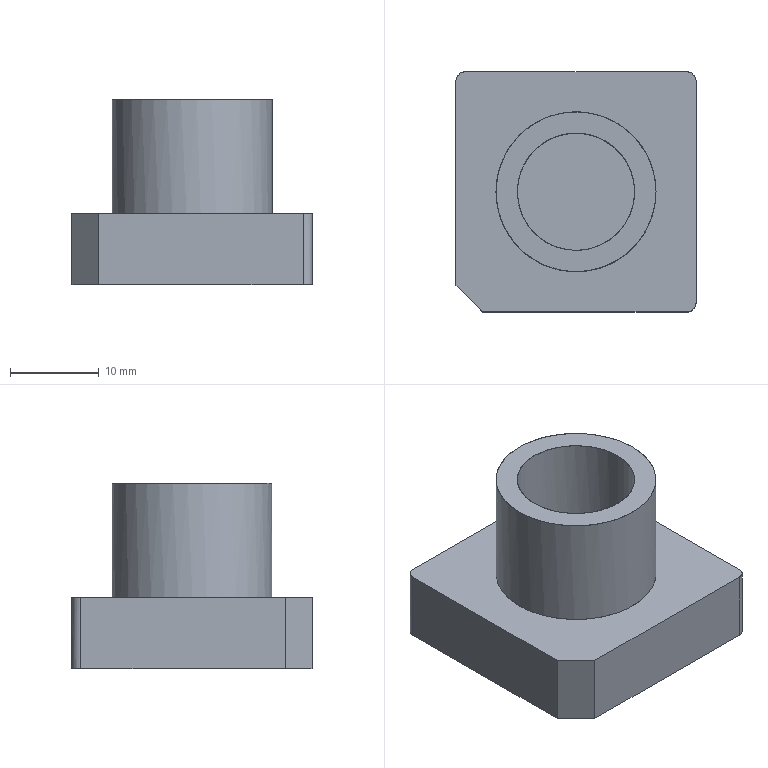NC program | PowerMill | posted with a generic post | part box 27 x 27 x 20.913 mm
Lines 16767 to 17771 of 92133:
N16864 M6
N16865 S18000 M03
N16866 G00 G90 X0.0 Y0.0
N16867 G43 Z10.803 H14
N16868
N16869 G05 P10000 R8
N16870 X-0.5036 Y-4.0685
N16871 Z0.9259
N16872 G01 Z-0.2741 F1200.0
N16873 X-0.499 Y-4.1188 F2000.0
N16874 X-0.4906 Y-4.1686
N16875 X-0.4782 Y-4.2176
N16876 X-0.4619 Y-4.2654
N16877 X-0.442 Y-4.3119
N16878 X-0.4184 Y-4.3566
N16879 X-0.3914 Y-4.3994
N16880 X-0.3611 Y-4.4398
N16881 X-0.3278 Y-4.4777
N16882 X-0.2915 Y-4.5129
N16883 X-0.2526 Y-4.5451
N16884 X-0.2112 Y-4.5741
N16885 X-0.1677 Y-4.5998
N16886 X-0.1223 Y-4.622
N16887 X-0.0753 Y-4.6405
N16888 X-0.0269 Y-4.6553
N16889 X0.0224 Y-4.6662
N16890 X0.0724 Y-4.6732
N16891 X0.1229 Y-4.6762
N16892 X0.1678 Y-4.6755
N16893 X0.3042 Y-4.6686
N16894 X0.4399 Y-4.6578
N16895 X0.5751 Y-4.6431
N16896 X0.7098 Y-4.6244
N16897 X0.8439 Y-4.6018
N16898 X0.9775 Y-4.5752
N16899 X1.1107 Y-4.5447
N16900 X1.2433 Y-4.5103
N16901 X1.3744 Y-4.4722
N16902 X1.504 Y-4.4304
N16903 X1.6321 Y-4.3849
N16904 X1.7586 Y-4.3357
N16905 X1.8838 Y-4.2828
N16906 X2.0074 Y-4.2262
N16907 X2.1296 Y-4.1658
N16908 X2.2504 Y-4.1017
N16909 X2.3698 Y-4.0338
N16910 X2.4859 Y-3.9634
N16911 X2.6001 Y-3.8896
N16912 X2.7121 Y-3.8123
N16913 X2.8221 Y-3.7317
N16914 X2.9297 Y-3.6477
N16915 X3.0351 Y-3.5606
N16916 X3.138 Y-3.4702
N16917 X3.2383 Y-3.3768
N16918 X3.336 Y-3.2804
N16919 X3.4271 Y-3.1851
N16920 X3.5154 Y-3.0873
N16921 X3.602 Y-2.9857
N16922 X3.6878 Y-2.8789
N16923 X3.7713 Y-2.7688
N16924 X3.8501 Y-2.6583
N16925 X3.9235 Y-2.5489
N16926 X3.9937 Y-2.4375
N16927 X4.0634 Y-2.3194
N16928 X4.1295 Y-2.1994
N16929 X4.1921 Y-2.0775
N16930 X4.2511 Y-1.9539
N16931 X4.3064 Y-1.8287
N16932 X4.3581 Y-1.7019
N16933 X4.406 Y-1.5738
N16934 X4.4501 Y-1.4444
N16935 X4.4904 Y-1.3139
N16936 X4.5268 Y-1.1823
N16937 X4.5593 Y-1.0497
N16938 X4.5879 Y-0.9167
N16939 X4.6126 Y-0.7825
N16940 X4.6335 Y-0.6472
N16941 X4.6505 Y-0.511
N16942 X4.6635 Y-0.3744
N16943 X4.6725 Y-0.2377
N16944 X4.6775 Y-0.1012
N16945 X4.6785 Y0.0348
N16946 X4.6755 Y0.17
N16947 X4.6686 Y0.305
N16948 X4.6576 Y0.4417
N16949 X4.6426 Y0.578
N16950 X4.6237 Y0.7137
N16951 X4.6009 Y0.8488
N16952 X4.5742 Y0.9828
N16953 X4.5436 Y1.1159
N16954 X4.5091 Y1.248
N16955 X4.4708 Y1.3791
N16956 X4.4286 Y1.5091
N16957 X4.3827 Y1.6378
N16958 X4.3329 Y1.7651
N16959 X4.2795 Y1.891
N16960 X4.2224 Y2.0152
N16961 X4.1617 Y2.1378
N16962 X4.0974 Y2.2585
N16963 X4.0297 Y2.3773
N16964 X3.9586 Y2.4938
N16965 X3.8841 Y2.6083
N16966 X3.8063 Y2.7205
N16967 X3.7252 Y2.8306
N16968 X3.6408 Y2.9383
N16969 X3.5533 Y3.0435
N16970 X3.4626 Y3.1463
N16971 X3.369 Y3.2464
N16972 X3.2723 Y3.3438
N16973 X3.1772 Y3.4344
N16974 X3.0795 Y3.5223
N16975 X2.9771 Y3.6091
N16976 X2.8699 Y3.6949
N16977 X2.76 Y3.7778
N16978 X2.6498 Y3.8559
N16979 X2.5406 Y3.9289
N16980 X2.4292 Y3.9986
N16981 X2.3103 Y4.0684
N16982 X2.1898 Y4.1345
N16983 X2.0678 Y4.1968
N16984 X1.9444 Y4.2555
N16985 X1.8195 Y4.3104
N16986 X1.6931 Y4.3616
N16987 X1.5654 Y4.409
N16988 X1.4363 Y4.4527
N16989 X1.3058 Y4.4927
N16990 X1.1741 Y4.5288
N16991 X1.041 Y4.5612
N16992 X0.9074 Y4.5897
N16993 X0.7728 Y4.6142
N16994 X0.6376 Y4.6349
N16995 X0.5019 Y4.6515
N16996 X0.3657 Y4.6642
N16997 X0.2293 Y4.6729
N16998 X0.0926 Y4.6776
N16999 X-0.0442 Y4.6783
N17000 X-0.1809 Y4.675
N17001 X-0.3175 Y4.6677
N17002 X-0.4538 Y4.6565
N17003 X-0.5897 Y4.6412
N17004 X-0.7251 Y4.622
N17005 X-0.8599 Y4.5988
N17006 X-0.9938 Y4.5717
N17007 X-1.1274 Y4.5406
N17008 X-1.2597 Y4.5058
N17009 X-1.3907 Y4.4672
N17010 X-1.5203 Y4.4248
N17011 X-1.6485 Y4.3787
N17012 X-1.7753 Y4.3288
N17013 X-1.9006 Y4.2753
N17014 X-2.0245 Y4.218
N17015 X-2.1468 Y4.157
N17016 X-2.2675 Y4.0923
N17017 X-2.3866 Y4.024
N17018 X-2.5027 Y3.9529
N17019 X-2.6166 Y3.8785
N17020 X-2.7285 Y3.8006
N17021 X-2.8382 Y3.7194
N17022 X-2.9456 Y3.635
N17023 X-3.0506 Y3.5473
N17024 X-3.1531 Y3.4565
N17025 X-3.253 Y3.3626
N17026 X-3.3503 Y3.2658
N17027 X-3.4409 Y3.1702
N17028 X-3.5288 Y3.072
N17029 X-3.6159 Y2.9688
N17030 X-3.7016 Y2.8613
N17031 X-3.784 Y2.7515
N17032 X-3.8619 Y2.6412
N17033 X-3.9347 Y2.5315
N17034 X-4.0043 Y2.4196
N17035 X-4.0739 Y2.3004
N17036 X-4.1397 Y2.1799
N17037 X-4.2017 Y2.058
N17038 X-4.26 Y1.9347
N17039 X-4.3145 Y1.8099
N17040 X-4.3653 Y1.6838
N17041 X-4.4123 Y1.5563
N17042 X-4.4556 Y1.4273
N17043 X-4.4952 Y1.2969
N17044 X-4.5311 Y1.165
N17045 X-4.5628 Y1.0335
N17046 X-4.5908 Y0.9014
N17047 X-4.615 Y0.7685
N17048 X-4.6354 Y0.6347
N17049 X-4.6517 Y0.5003
N17050 X-4.6642 Y0.3656
N17051 X-4.6727 Y0.2308
N17052 X-4.6775 Y0.0953
N17053 X-4.6783 Y-0.0414
N17054 X-4.6752 Y-0.1778
N17055 X-4.6681 Y-0.3138
N17056 X-4.657 Y-0.4494
N17057 X-4.6419 Y-0.5846
N17058 X-4.6229 Y-0.7196
N17059 X-4.5998 Y-0.8542
N17060 X-4.5728 Y-0.9885
N17061 X-4.5418 Y-1.1222
N17062 X-4.5071 Y-1.2546
N17063 X-4.4688 Y-1.3855
N17064 X-4.4267 Y-1.5149
N17065 X-4.3809 Y-1.6428
N17066 X-4.3314 Y-1.7693
N17067 X-4.2781 Y-1.8944
N17068 X-4.2211 Y-2.018
N17069 X-4.1604 Y-2.1401
N17070 X-4.0959 Y-2.2609
N17071 X-4.0277 Y-2.3803
N17072 X-3.957 Y-2.4962
N17073 X-3.8828 Y-2.6102
N17074 X-3.8052 Y-2.7221
N17075 X-3.7243 Y-2.8318
N17076 X-3.6401 Y-2.9393
N17077 X-3.5526 Y-3.0444
N17078 X-3.462 Y-3.147
N17079 X-3.3683 Y-3.2471
N17080 X-3.2716 Y-3.3445
N17081 X-3.1758 Y-3.4357
N17082 X-3.0774 Y-3.5241
N17083 X-2.9748 Y-3.611
N17084 X-2.8675 Y-3.6967
N17085 X-2.7573 Y-3.7797
N17086 X-2.6468 Y-3.8581
N17087 X-2.5367 Y-3.9314
N17088 X-2.4246 Y-4.0015
N17089 X-2.3063 Y-4.0708
N17090 X-2.1861 Y-4.1365
N17091 X-2.0641 Y-4.1987
N17092 X-1.9403 Y-4.2573
N17093 X-1.8149 Y-4.3123
N17094 X-1.6881 Y-4.3635
N17095 X-1.5598 Y-4.411
N17096 X-1.4303 Y-4.4546
N17097 X-1.2997 Y-4.4945
N17098 X-1.168 Y-4.5305
N17099 X-1.0353 Y-4.5626
N17100 X-0.9018 Y-4.5908
N17101 X-0.767 Y-4.6152
N17102 X-0.6316 Y-4.6357
N17103 X-0.4957 Y-4.6522
N17104 X-0.3595 Y-4.6647
N17105 X-0.223 Y-4.6732
N17106 X-0.0863 Y-4.6777
N17107 X0.0503 Y-4.6782
N17108 X0.1678 Y-4.6755
N17109 X0.2182 Y-4.6723
N17110 X0.2683 Y-4.6652
N17111 X0.3176 Y-4.6541
N17112 X0.3658 Y-4.6392
N17113 X0.4128 Y-4.6205
N17114 X0.4582 Y-4.5981
N17115 X0.5016 Y-4.5723
N17116 X0.5428 Y-4.5431
N17117 X0.5816 Y-4.5108
N17118 X0.6178 Y-4.4754
N17119 X0.651 Y-4.4374
N17120 X0.6812 Y-4.3969
N17121 X0.708 Y-4.3541
N17122 X0.7314 Y-4.3093
N17123 X0.7512 Y-4.2627
N17124 X0.7673 Y-4.2148
N17125 X0.7795 Y-4.1658
N17126 X0.7878 Y-4.116
N17127 X0.7921 Y-4.0656
N17128 X0.7927 Y-4.0207
N17129 X-0.5036 Y-4.0685 Z-0.314
N17130 X-0.499 Y-4.1188
N17131 X-0.4906 Y-4.1686
N17132 X-0.4782 Y-4.2176
N17133 X-0.4619 Y-4.2654
N17134 X-0.442 Y-4.3119
N17135 X-0.4184 Y-4.3566
N17136 X-0.3914 Y-4.3994
N17137 X-0.3611 Y-4.4398
N17138 X-0.3278 Y-4.4777
N17139 X-0.2915 Y-4.5129
N17140 X-0.2526 Y-4.5451
N17141 X-0.2112 Y-4.5741
N17142 X-0.1677 Y-4.5998
N17143 X-0.1223 Y-4.622
N17144 X-0.0753 Y-4.6405
N17145 X-0.0269 Y-4.6553
N17146 X0.0224 Y-4.6662
N17147 X0.0724 Y-4.6732
N17148 X0.1229 Y-4.6762
N17149 X0.1678 Y-4.6755
N17150 X0.3042 Y-4.6686
N17151 X0.4399 Y-4.6578
N17152 X0.5751 Y-4.6431
N17153 X0.7098 Y-4.6244
N17154 X0.8439 Y-4.6018
N17155 X0.9775 Y-4.5752
N17156 X1.1107 Y-4.5447
N17157 X1.2433 Y-4.5103
N17158 X1.3744 Y-4.4722
N17159 X1.504 Y-4.4304
N17160 X1.6321 Y-4.3849
N17161 X1.7586 Y-4.3357
N17162 X1.8838 Y-4.2828
N17163 X2.0074 Y-4.2262
N17164 X2.1296 Y-4.1658
N17165 X2.2504 Y-4.1017
N17166 X2.3698 Y-4.0338
N17167 X2.4859 Y-3.9634
N17168 X2.6001 Y-3.8896
N17169 X2.7121 Y-3.8123
N17170 X2.8221 Y-3.7317
N17171 X2.9297 Y-3.6477
N17172 X3.0351 Y-3.5606
N17173 X3.138 Y-3.4702
N17174 X3.2383 Y-3.3768
N17175 X3.336 Y-3.2803
N17176 X3.4271 Y-3.1851
N17177 X3.5154 Y-3.0873
N17178 X3.602 Y-2.9857
N17179 X3.6878 Y-2.8789
N17180 X3.7713 Y-2.7688
N17181 X3.8501 Y-2.6583
N17182 X3.9235 Y-2.5489
N17183 X3.9937 Y-2.4375
N17184 X4.0634 Y-2.3194
N17185 X4.1295 Y-2.1994
N17186 X4.1921 Y-2.0775
N17187 X4.2511 Y-1.9539
N17188 X4.3064 Y-1.8287
N17189 X4.3581 Y-1.7019
N17190 X4.406 Y-1.5738
N17191 X4.4501 Y-1.4444
N17192 X4.4904 Y-1.3139
N17193 X4.5268 Y-1.1823
N17194 X4.5593 Y-1.0497
N17195 X4.5879 Y-0.9167
N17196 X4.6126 Y-0.7825
N17197 X4.6335 Y-0.6472
N17198 X4.6505 Y-0.511
N17199 X4.6635 Y-0.3744
N17200 X4.6725 Y-0.2377
N17201 X4.6775 Y-0.1012
N17202 X4.6785 Y0.0348
N17203 X4.6755 Y0.17
N17204 X4.6686 Y0.305
N17205 X4.6576 Y0.4417
N17206 X4.6426 Y0.578
N17207 X4.6237 Y0.7137
N17208 X4.6009 Y0.8488
N17209 X4.5742 Y0.9828
N17210 X4.5436 Y1.1159
N17211 X4.5091 Y1.248
N17212 X4.4708 Y1.3791
N17213 X4.4286 Y1.5091
N17214 X4.3827 Y1.6378
N17215 X4.3329 Y1.7651
N17216 X4.2795 Y1.891
N17217 X4.2224 Y2.0152
N17218 X4.1617 Y2.1378
N17219 X4.0974 Y2.2585
N17220 X4.0297 Y2.3773
N17221 X3.9586 Y2.4938
N17222 X3.8841 Y2.6083
N17223 X3.8063 Y2.7205
N17224 X3.7252 Y2.8306
N17225 X3.6408 Y2.9383
N17226 X3.5533 Y3.0435
N17227 X3.4626 Y3.1463
N17228 X3.369 Y3.2464
N17229 X3.2723 Y3.3438
N17230 X3.1772 Y3.4345
N17231 X3.0795 Y3.5223
N17232 X2.9771 Y3.6091
N17233 X2.8699 Y3.6949
N17234 X2.76 Y3.7778
N17235 X2.6498 Y3.856
N17236 X2.5405 Y3.9289
N17237 X2.4292 Y3.9986
N17238 X2.3102 Y4.0684
N17239 X2.1898 Y4.1345
N17240 X2.0678 Y4.1969
N17241 X1.9443 Y4.2555
N17242 X1.8194 Y4.3104
N17243 X1.6931 Y4.3616
N17244 X1.5654 Y4.4091
N17245 X1.4363 Y4.4527
N17246 X1.3058 Y4.4927
N17247 X1.174 Y4.5288
N17248 X1.0409 Y4.5612
N17249 X0.9073 Y4.5897
N17250 X0.7728 Y4.6142
N17251 X0.6376 Y4.6349
N17252 X0.5019 Y4.6515
N17253 X0.3657 Y4.6642
N17254 X0.2292 Y4.6729
N17255 X0.0925 Y4.6776
N17256 X-0.0442 Y4.6783
N17257 X-0.1809 Y4.675
N17258 X-0.3175 Y4.6677
N17259 X-0.4538 Y4.6565
N17260 X-0.5897 Y4.6412
N17261 X-0.7251 Y4.622
N17262 X-0.8599 Y4.5988
N17263 X-0.9938 Y4.5717
N17264 X-1.1274 Y4.5406
N17265 X-1.2597 Y4.5058
N17266 X-1.3907 Y4.4672
N17267 X-1.5204 Y4.4248
N17268 X-1.6486 Y4.3787
N17269 X-1.7754 Y4.3288
N17270 X-1.9007 Y4.2752
N17271 X-2.0245 Y4.218
N17272 X-2.1468 Y4.157
N17273 X-2.2675 Y4.0923
N17274 X-2.3867 Y4.024
N17275 X-2.5027 Y3.9529
N17276 X-2.6167 Y3.8785
N17277 X-2.7285 Y3.8006
N17278 X-2.8382 Y3.7194
N17279 X-2.9456 Y3.6349
N17280 X-3.0506 Y3.5473
N17281 X-3.1531 Y3.4564
N17282 X-3.253 Y3.3626
N17283 X-3.3503 Y3.2658
N17284 X-3.4409 Y3.1702
N17285 X-3.5288 Y3.072
N17286 X-3.616 Y2.9688
N17287 X-3.7016 Y2.8613
N17288 X-3.784 Y2.7514
N17289 X-3.8619 Y2.6412
N17290 X-3.9347 Y2.5314
N17291 X-4.0044 Y2.4196
N17292 X-4.0739 Y2.3004
N17293 X-4.1397 Y2.1799
N17294 X-4.2017 Y2.0579
N17295 X-4.26 Y1.9346
N17296 X-4.3145 Y1.8099
N17297 X-4.3653 Y1.6838
N17298 X-4.4123 Y1.5562
N17299 X-4.4556 Y1.4273
N17300 X-4.4952 Y1.2969
N17301 X-4.5311 Y1.165
N17302 X-4.5628 Y1.0335
N17303 X-4.5908 Y0.9014
N17304 X-4.615 Y0.7684
N17305 X-4.6354 Y0.6346
N17306 X-4.6517 Y0.5003
N17307 X-4.6642 Y0.3656
N17308 X-4.6727 Y0.2307
N17309 X-4.6775 Y0.0953
N17310 X-4.6783 Y-0.0414
N17311 X-4.6752 Y-0.1778
N17312 X-4.6681 Y-0.3138
N17313 X-4.657 Y-0.4494
N17314 X-4.6419 Y-0.5847
N17315 X-4.6229 Y-0.7196
N17316 X-4.5998 Y-0.8542
N17317 X-4.5728 Y-0.9885
N17318 X-4.5418 Y-1.1223
N17319 X-4.5071 Y-1.2546
N17320 X-4.4688 Y-1.3855
N17321 X-4.4267 Y-1.5149
N17322 X-4.3809 Y-1.6428
N17323 X-4.3313 Y-1.7693
N17324 X-4.2781 Y-1.8944
N17325 X-4.2211 Y-2.018
N17326 X-4.1604 Y-2.1402
N17327 X-4.0959 Y-2.2609
N17328 X-4.0277 Y-2.3803
N17329 X-3.957 Y-2.4962
N17330 X-3.8828 Y-2.6102
N17331 X-3.8052 Y-2.7221
N17332 X-3.7243 Y-2.8318
N17333 X-3.6401 Y-2.9393
N17334 X-3.5526 Y-3.0444
N17335 X-3.462 Y-3.147
N17336 X-3.3683 Y-3.2471
N17337 X-3.2716 Y-3.3446
N17338 X-3.1758 Y-3.4357
N17339 X-3.0774 Y-3.5241
N17340 X-2.9748 Y-3.611
N17341 X-2.8675 Y-3.6967
N17342 X-2.7573 Y-3.7797
N17343 X-2.6467 Y-3.8581
N17344 X-2.5367 Y-3.9314
N17345 X-2.4245 Y-4.0016
N17346 X-2.3063 Y-4.0708
N17347 X-2.1861 Y-4.1366
N17348 X-2.064 Y-4.1988
N17349 X-1.9403 Y-4.2574
N17350 X-1.8149 Y-4.3123
N17351 X-1.688 Y-4.3635
N17352 X-1.5598 Y-4.411
N17353 X-1.4303 Y-4.4546
N17354 X-1.2997 Y-4.4945
N17355 X-1.168 Y-4.5305
N17356 X-1.0353 Y-4.5626
N17357 X-0.9017 Y-4.5908
N17358 X-0.767 Y-4.6152
N17359 X-0.6316 Y-4.6357
N17360 X-0.4957 Y-4.6522
N17361 X-0.3594 Y-4.6647
N17362 X-0.2229 Y-4.6732
N17363 X-0.0863 Y-4.6777
N17364 X0.0504 Y-4.6782
N17365 X0.1678 Y-4.6755
N17366 X0.2182 Y-4.6723
N17367 X0.2683 Y-4.6652
N17368 X0.3176 Y-4.6541
N17369 X0.3658 Y-4.6392
N17370 X0.4128 Y-4.6205
N17371 X0.4582 Y-4.5981
N17372 X0.5016 Y-4.5723
N17373 X0.5428 Y-4.5431
N17374 X0.5816 Y-4.5108
N17375 X0.6178 Y-4.4754
N17376 X0.651 Y-4.4374
N17377 X0.6812 Y-4.3969
N17378 X0.708 Y-4.3541
N17379 X0.7314 Y-4.3093
N17380 X0.7512 Y-4.2627
N17381 X0.7672 Y-4.2148
N17382 X0.7795 Y-4.1658
N17383 X0.7878 Y-4.116
N17384 X0.7921 Y-4.0656
N17385 X0.7927 Y-4.0207
N17386 X-0.5036 Y-4.0685 Z-0.3539
N17387 X-0.499 Y-4.1188
N17388 X-0.4906 Y-4.1686
N17389 X-0.4782 Y-4.2176
N17390 X-0.4619 Y-4.2654
N17391 X-0.442 Y-4.3119
N17392 X-0.4184 Y-4.3566
N17393 X-0.3914 Y-4.3994
N17394 X-0.3611 Y-4.4398
N17395 X-0.3278 Y-4.4777
N17396 X-0.2915 Y-4.5129
N17397 X-0.2526 Y-4.5451
N17398 X-0.2112 Y-4.5741
N17399 X-0.1677 Y-4.5998
N17400 X-0.1223 Y-4.622
N17401 X-0.0753 Y-4.6405
N17402 X-0.0269 Y-4.6553
N17403 X0.0224 Y-4.6662
N17404 X0.0724 Y-4.6732
N17405 X0.1229 Y-4.6762
N17406 X0.1678 Y-4.6755
N17407 X0.3042 Y-4.6686
N17408 X0.4399 Y-4.6578
N17409 X0.5751 Y-4.6431
N17410 X0.7098 Y-4.6244
N17411 X0.8439 Y-4.6018
N17412 X0.9775 Y-4.5752
N17413 X1.1107 Y-4.5447
N17414 X1.2433 Y-4.5103
N17415 X1.3744 Y-4.4722
N17416 X1.504 Y-4.4304
N17417 X1.6321 Y-4.3849
N17418 X1.7587 Y-4.3357
N17419 X1.8838 Y-4.2828
N17420 X2.0074 Y-4.2262
N17421 X2.1296 Y-4.1658
N17422 X2.2504 Y-4.1017
N17423 X2.3699 Y-4.0338
N17424 X2.4859 Y-3.9634
N17425 X2.6001 Y-3.8896
N17426 X2.7122 Y-3.8123
N17427 X2.8221 Y-3.7317
N17428 X2.9298 Y-3.6477
N17429 X3.0351 Y-3.5606
N17430 X3.138 Y-3.4702
N17431 X3.2383 Y-3.3768
N17432 X3.336 Y-3.2803
N17433 X3.4271 Y-3.1851
N17434 X3.5154 Y-3.0873
N17435 X3.602 Y-2.9857
N17436 X3.6878 Y-2.8789
N17437 X3.7713 Y-2.7688
N17438 X3.8501 Y-2.6583
N17439 X3.9235 Y-2.5489
N17440 X3.9937 Y-2.4374
N17441 X4.0634 Y-2.3194
N17442 X4.1295 Y-2.1994
N17443 X4.1921 Y-2.0775
N17444 X4.2511 Y-1.9539
N17445 X4.3065 Y-1.8287
N17446 X4.3581 Y-1.7019
N17447 X4.406 Y-1.5738
N17448 X4.4501 Y-1.4444
N17449 X4.4904 Y-1.3139
N17450 X4.5268 Y-1.1823
N17451 X4.5593 Y-1.0496
N17452 X4.5879 Y-0.9167
N17453 X4.6126 Y-0.7825
N17454 X4.6335 Y-0.6472
N17455 X4.6505 Y-0.511
N17456 X4.6635 Y-0.3744
N17457 X4.6725 Y-0.2377
N17458 X4.6775 Y-0.1012
N17459 X4.6785 Y0.0348
N17460 X4.6755 Y0.17
N17461 X4.6686 Y0.305
N17462 X4.6576 Y0.4417
N17463 X4.6426 Y0.578
N17464 X4.6237 Y0.7137
N17465 X4.6009 Y0.8488
N17466 X4.5742 Y0.9828
N17467 X4.5436 Y1.1159
N17468 X4.5091 Y1.248
N17469 X4.4708 Y1.3791
N17470 X4.4286 Y1.5091
N17471 X4.3827 Y1.6378
N17472 X4.3329 Y1.7651
N17473 X4.2795 Y1.891
N17474 X4.2224 Y2.0152
N17475 X4.1617 Y2.1378
N17476 X4.0974 Y2.2585
N17477 X4.0297 Y2.3773
N17478 X3.9586 Y2.4938
N17479 X3.8841 Y2.6083
N17480 X3.8063 Y2.7205
N17481 X3.7252 Y2.8306
N17482 X3.6408 Y2.9383
N17483 X3.5533 Y3.0435
N17484 X3.4626 Y3.1463
N17485 X3.369 Y3.2464
N17486 X3.2723 Y3.3438
N17487 X3.1772 Y3.4345
N17488 X3.0795 Y3.5223
N17489 X2.9771 Y3.6091
N17490 X2.8699 Y3.6949
N17491 X2.7599 Y3.7778
N17492 X2.6498 Y3.856
N17493 X2.5405 Y3.9289
N17494 X2.4291 Y3.9987
N17495 X2.3102 Y4.0684
N17496 X2.1897 Y4.1345
N17497 X2.0678 Y4.1969
N17498 X1.9443 Y4.2555
N17499 X1.8194 Y4.3104
N17500 X1.6931 Y4.3616
N17501 X1.5653 Y4.4091
N17502 X1.4362 Y4.4528
N17503 X1.3058 Y4.4927
N17504 X1.174 Y4.5288
N17505 X1.0409 Y4.5612
N17506 X0.9073 Y4.5897
N17507 X0.7728 Y4.6142
N17508 X0.6376 Y4.6349
N17509 X0.5018 Y4.6515
N17510 X0.3657 Y4.6642
N17511 X0.2292 Y4.6729
N17512 X0.0925 Y4.6776
N17513 X-0.0443 Y4.6783
N17514 X-0.181 Y4.675
N17515 X-0.3175 Y4.6677
N17516 X-0.4538 Y4.6564
N17517 X-0.5897 Y4.6412
N17518 X-0.7251 Y4.622
N17519 X-0.8599 Y4.5988
N17520 X-0.9938 Y4.5717
N17521 X-1.1274 Y4.5406
N17522 X-1.2598 Y4.5058
N17523 X-1.3908 Y4.4672
N17524 X-1.5204 Y4.4248
N17525 X-1.6486 Y4.3787
N17526 X-1.7754 Y4.3288
N17527 X-1.9007 Y4.2752
N17528 X-2.0245 Y4.2179
N17529 X-2.1468 Y4.157
N17530 X-2.2676 Y4.0923
N17531 X-2.3867 Y4.024
N17532 X-2.5027 Y3.9529
N17533 X-2.6167 Y3.8784
N17534 X-2.7286 Y3.8006
N17535 X-2.8383 Y3.7194
N17536 X-2.9456 Y3.6349
N17537 X-3.0506 Y3.5472
N17538 X-3.1531 Y3.4564
N17539 X-3.2531 Y3.3626
N17540 X-3.3503 Y3.2657
N17541 X-3.441 Y3.1701
N17542 X-3.5288 Y3.072
N17543 X-3.616 Y2.9687
N17544 X-3.7016 Y2.8612
N17545 X-3.784 Y2.7514
N17546 X-3.8619 Y2.6412
N17547 X-3.9348 Y2.5314
N17548 X-4.0044 Y2.4196
N17549 X-4.0739 Y2.3004
N17550 X-4.1397 Y2.1798
N17551 X-4.2017 Y2.0579
N17552 X-4.26 Y1.9346
N17553 X-4.3145 Y1.8099
N17554 X-4.3653 Y1.6838
N17555 X-4.4123 Y1.5562
N17556 X-4.4556 Y1.4272
N17557 X-4.4952 Y1.2968
N17558 X-4.5311 Y1.165
N17559 X-4.5629 Y1.0334
N17560 X-4.5908 Y0.9013
N17561 X-4.615 Y0.7684
N17562 X-4.6354 Y0.6346
N17563 X-4.6518 Y0.5002
N17564 X-4.6642 Y0.3656
N17565 X-4.6727 Y0.2307
N17566 X-4.6775 Y0.0953
N17567 X-4.6783 Y-0.0415
N17568 X-4.6752 Y-0.1778
N17569 X-4.6681 Y-0.3138
N17570 X-4.657 Y-0.4494
N17571 X-4.6419 Y-0.5847
N17572 X-4.6229 Y-0.7196
N17573 X-4.5998 Y-0.8542
N17574 X-4.5728 Y-0.9885
N17575 X-4.5418 Y-1.1223
N17576 X-4.5071 Y-1.2547
N17577 X-4.4687 Y-1.3855
N17578 X-4.4267 Y-1.5149
N17579 X-4.3809 Y-1.6429
N17580 X-4.3313 Y-1.7694
N17581 X-4.2781 Y-1.8944
N17582 X-4.2211 Y-2.018
N17583 X-4.1604 Y-2.1402
N17584 X-4.0959 Y-2.261
N17585 X-4.0277 Y-2.3803
N17586 X-3.9569 Y-2.4962
N17587 X-3.8828 Y-2.6102
N17588 X-3.8052 Y-2.7221
N17589 X-3.7243 Y-2.8318
N17590 X-3.64 Y-2.9393
N17591 X-3.5526 Y-3.0444
N17592 X-3.462 Y-3.1471
N17593 X-3.3683 Y-3.2472
N17594 X-3.2716 Y-3.3446
N17595 X-3.1758 Y-3.4358
N17596 X-3.0773 Y-3.5241
N17597 X-2.9747 Y-3.6111
N17598 X-2.8674 Y-3.6968
N17599 X-2.7572 Y-3.7797
N17600 X-2.6467 Y-3.8581
N17601 X-2.5366 Y-3.9315
N17602 X-2.4245 Y-4.0016
N17603 X-2.3062 Y-4.0708
N17604 X-2.186 Y-4.1366
N17605 X-2.064 Y-4.1988
N17606 X-1.9402 Y-4.2574
N17607 X-1.8148 Y-4.3123
N17608 X-1.6879 Y-4.3635
N17609 X-1.5597 Y-4.411
N17610 X-1.4302 Y-4.4547
N17611 X-1.2996 Y-4.4945
N17612 X-1.1679 Y-4.5305
N17613 X-1.0352 Y-4.5626
N17614 X-0.9017 Y-4.5908
N17615 X-0.7669 Y-4.6152
N17616 X-0.6315 Y-4.6357
N17617 X-0.4956 Y-4.6522
N17618 X-0.3593 Y-4.6647
N17619 X-0.2228 Y-4.6732
N17620 X-0.0862 Y-4.6777
N17621 X0.0504 Y-4.6782
N17622 X0.1678 Y-4.6755
N17623 X0.2182 Y-4.6723
N17624 X0.2683 Y-4.6652
N17625 X0.3176 Y-4.6541
N17626 X0.3658 Y-4.6392
N17627 X0.4128 Y-4.6205
N17628 X0.4582 Y-4.5981
N17629 X0.5016 Y-4.5723
N17630 X0.5428 Y-4.5431
N17631 X0.5816 Y-4.5107
N17632 X0.6178 Y-4.4754
N17633 X0.651 Y-4.4374
N17634 X0.6812 Y-4.3969
N17635 X0.708 Y-4.3541
N17636 X0.7314 Y-4.3093
N17637 X0.7512 Y-4.2627
N17638 X0.7672 Y-4.2148
N17639 X0.7795 Y-4.1658
N17640 X0.7878 Y-4.116
N17641 X0.7921 Y-4.0656
N17642 X0.7927 Y-4.0207
N17643 X-0.5036 Y-4.0685 Z-0.3938
N17644 X-0.499 Y-4.1188
N17645 X-0.4906 Y-4.1686
N17646 X-0.4782 Y-4.2176
N17647 X-0.4619 Y-4.2654
N17648 X-0.442 Y-4.3119
N17649 X-0.4184 Y-4.3566
N17650 X-0.3914 Y-4.3994
N17651 X-0.3611 Y-4.4398
N17652 X-0.3278 Y-4.4777
N17653 X-0.2915 Y-4.5129
N17654 X-0.2526 Y-4.5451
N17655 X-0.2112 Y-4.5741
N17656 X-0.1677 Y-4.5998
N17657 X-0.1223 Y-4.622
N17658 X-0.0753 Y-4.6405
N17659 X-0.0269 Y-4.6553
N17660 X0.0224 Y-4.6662
N17661 X0.0724 Y-4.6732
N17662 X0.1229 Y-4.6762
N17663 X0.1678 Y-4.6755
N17664 X0.3042 Y-4.6686
N17665 X0.4399 Y-4.6578
N17666 X0.5751 Y-4.6431
N17667 X0.7098 Y-4.6244
N17668 X0.8439 Y-4.6018
N17669 X0.9775 Y-4.5752
N17670 X1.1107 Y-4.5447
N17671 X1.2433 Y-4.5103
N17672 X1.3744 Y-4.4722
N17673 X1.504 Y-4.4304
N17674 X1.6321 Y-4.3849
N17675 X1.7587 Y-4.3357
N17676 X1.8838 Y-4.2828
N17677 X2.0074 Y-4.2262
N17678 X2.1296 Y-4.1658
N17679 X2.2504 Y-4.1017
N17680 X2.3699 Y-4.0338
N17681 X2.4859 Y-3.9634
N17682 X2.6001 Y-3.8896
N17683 X2.7122 Y-3.8123
N17684 X2.8221 Y-3.7317
N17685 X2.9298 Y-3.6477
N17686 X3.0351 Y-3.5605
N17687 X3.138 Y-3.4702
N17688 X3.2383 Y-3.3768
N17689 X3.336 Y-3.2803
N17690 X3.4271 Y-3.1851
N17691 X3.5154 Y-3.0873
N17692 X3.602 Y-2.9857
N17693 X3.6878 Y-2.8789
N17694 X3.7713 Y-2.7688
N17695 X3.8501 Y-2.6583
N17696 X3.9235 Y-2.5489
N17697 X3.9937 Y-2.4374
N17698 X4.0634 Y-2.3194
N17699 X4.1295 Y-2.1994
N17700 X4.1921 Y-2.0775
N17701 X4.2511 Y-1.9539
N17702 X4.3065 Y-1.8287
N17703 X4.3581 Y-1.7019
N17704 X4.406 Y-1.5738
N17705 X4.4501 Y-1.4444
N17706 X4.4904 Y-1.3139
N17707 X4.5268 Y-1.1823
N17708 X4.5594 Y-1.0496
N17709 X4.5879 Y-0.9167
N17710 X4.6126 Y-0.7825
N17711 X4.6335 Y-0.6472
N17712 X4.6505 Y-0.511
N17713 X4.6635 Y-0.3744
N17714 X4.6725 Y-0.2377
N17715 X4.6775 Y-0.1012
N17716 X4.6785 Y0.0348
N17717 X4.6755 Y0.17
N17718 X4.6686 Y0.305
N17719 X4.6576 Y0.4417
N17720 X4.6426 Y0.578
N17721 X4.6237 Y0.7138
N17722 X4.6009 Y0.8488
N17723 X4.5742 Y0.9828
N17724 X4.5436 Y1.1159
N17725 X4.5091 Y1.2481
N17726 X4.4708 Y1.3792
N17727 X4.4286 Y1.5091
N17728 X4.3827 Y1.6378
N17729 X4.3329 Y1.7651
N17730 X4.2795 Y1.891
N17731 X4.2224 Y2.0153
N17732 X4.1617 Y2.1378
N17733 X4.0974 Y2.2585
N17734 X4.0297 Y2.3773
N17735 X3.9586 Y2.4939
N17736 X3.8841 Y2.6083
N17737 X3.8063 Y2.7205
N17738 X3.7252 Y2.8306
N17739 X3.6408 Y2.9383
N17740 X3.5533 Y3.0435
N17741 X3.4626 Y3.1463
N17742 X3.3689 Y3.2464
N17743 X3.2723 Y3.3439
N17744 X3.1772 Y3.4345
N17745 X3.0794 Y3.5223
N17746 X2.977 Y3.6092
N17747 X2.8698 Y3.6949
N17748 X2.7599 Y3.7778
N17749 X2.6498 Y3.856
N17750 X2.5405 Y3.9289
N17751 X2.4291 Y3.9987
N17752 X2.3102 Y4.0684
N17753 X2.1897 Y4.1345
N17754 X2.0677 Y4.1969
N17755 X1.9443 Y4.2555
N17756 X1.8194 Y4.3105
N17757 X1.693 Y4.3616
N17758 X1.5653 Y4.4091
N17759 X1.4362 Y4.4528
N17760 X1.3057 Y4.4927
N17761 X1.174 Y4.5288
N17762 X1.0409 Y4.5612
N17763 X0.9073 Y4.5897
N17764 X0.7727 Y4.6142
N17765 X0.6376 Y4.6349
N17766 X0.5018 Y4.6515
N17767 X0.3656 Y4.6642
N17768 X0.2292 Y4.6729
N17769 X0.0925 Y4.6776
N17770 X-0.0443 Y4.6783
N17771 X-0.181 Y4.675
N17772 X-0.3176 Y4.6677
N17773 X-0.4539 Y4.6564
N17774 X-0.5898 Y4.6412
N17775 X-0.7252 Y4.622
N17776 X-0.86 Y4.5988
N17777 X-0.9938 Y4.5717
N17778 X-1.1275 Y4.5406
N17779 X-1.2598 Y4.5058
N17780 X-1.3908 Y4.4671
N17781 X-1.5204 Y4.4248
N17782 X-1.6486 Y4.3786
N17783 X-1.7754 Y4.3288
N17784 X-1.9007 Y4.2752
N17785 X-2.0245 Y4.2179
N17786 X-2.1468 Y4.157
N17787 X-2.2676 Y4.0923
N17788 X-2.3867 Y4.0239
N17789 X-2.5027 Y3.9529
N17790 X-2.6167 Y3.8784
N17791 X-2.7286 Y3.8006
N17792 X-2.8383 Y3.7194
N17793 X-2.9457 Y3.6349
N17794 X-3.0507 Y3.5472
N17795 X-3.1532 Y3.4564
N17796 X-3.2531 Y3.3625
N17797 X-3.3503 Y3.2657
N17798 X-3.441 Y3.1701
N17799 X-3.5288 Y3.0719
N17800 X-3.616 Y2.9687
N17801 X-3.7016 Y2.8612
N17802 X-3.784 Y2.7514
N17803 X-3.8619 Y2.6411
N17804 X-3.9348 Y2.5314
N17805 X-4.0044 Y2.4195
N17806 X-4.074 Y2.3004
N17807 X-4.1397 Y2.1798
N17808 X-4.2018 Y2.0579
N17809 X-4.26 Y1.9346
N17810 X-4.3145 Y1.8098
N17811 X-4.3653 Y1.6837
N17812 X-4.4123 Y1.5562
N17813 X-4.4556 Y1.4272
N17814 X-4.4952 Y1.2968
N17815 X-4.5311 Y1.1649
N17816 X-4.5629 Y1.0334
N17817 X-4.5908 Y0.9013
N17818 X-4.615 Y0.7684
N17819 X-4.6354 Y0.6346
N17820 X-4.6518 Y0.5002
N17821 X-4.6642 Y0.3655
N17822 X-4.6727 Y0.2307
N17823 X-4.6775 Y0.0952
N17824 X-4.6783 Y-0.0415
N17825 X-4.6752 Y-0.1779
N17826 X-4.6681 Y-0.3139
N17827 X-4.657 Y-0.4495
N17828 X-4.6419 Y-0.5847
N17829 X-4.6228 Y-0.7197
N17830 X-4.5998 Y-0.8543
N17831 X-4.5728 Y-0.9886
N17832 X-4.5418 Y-1.1223
N17833 X-4.5071 Y-1.2547
N17834 X-4.4687 Y-1.3856
N17835 X-4.4266 Y-1.515
N17836 X-4.3808 Y-1.6429
N17837 X-4.3313 Y-1.7694
N17838 X-4.2781 Y-1.8945
N17839 X-4.2211 Y-2.0181
N17840 X-4.1603 Y-2.1402
N17841 X-4.0959 Y-2.261
N17842 X-4.0276 Y-2.3804
N17843 X-3.9569 Y-2.4963
N17844 X-3.8827 Y-2.6103
N17845 X-3.8052 Y-2.7222
N17846 X-3.7242 Y-2.8319
N17847 X-3.64 Y-2.9393
N17848 X-3.5525 Y-3.0445
N17849 X-3.4619 Y-3.1471
N17850 X-3.3682 Y-3.2472
N17851 X-3.2716 Y-3.3446
N17852 X-3.1757 Y-3.4358
N17853 X-3.0773 Y-3.5242
N17854 X-2.9747 Y-3.6111
N17855 X-2.8674 Y-3.6968
N17856 X-2.7572 Y-3.7798
N17857 X-2.6466 Y-3.8582
N17858 X-2.5366 Y-3.9315
N17859 X-2.4244 Y-4.0016
N17860 X-2.3061 Y-4.0709
N17861 X-2.1859 Y-4.1366
N17862 X-2.0639 Y-4.1988
N17863 X-1.9401 Y-4.2574
N17864 X-1.8147 Y-4.3123
N17865 X-1.6879 Y-4.3636
N17866 X-1.5596 Y-4.411
N17867 X-1.4302 Y-4.4547
N17868 X-1.2995 Y-4.4945